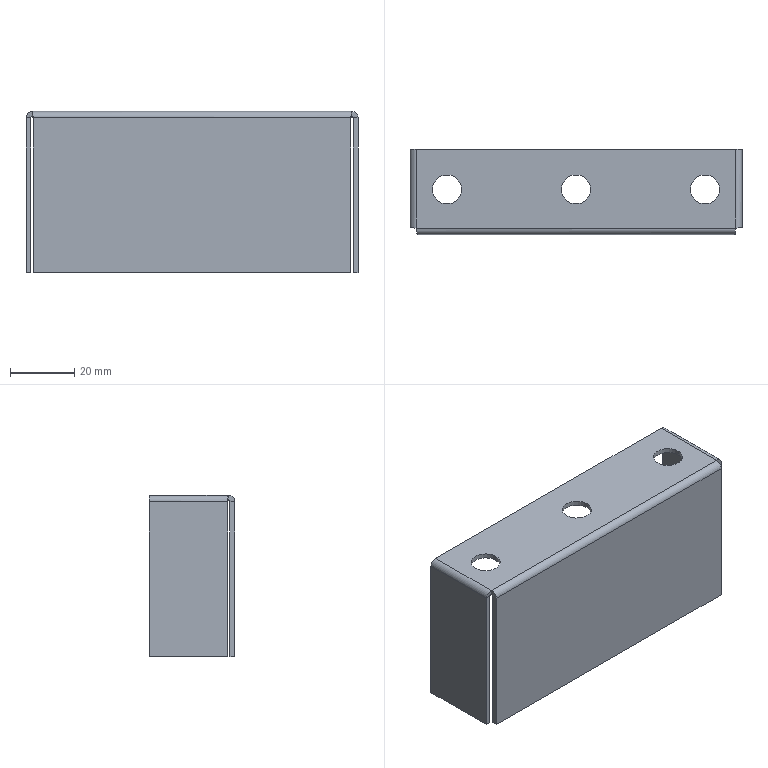Part | SolidWorks | features BaseBody 1 | 1 solid | 36 faces | box 103 x 26.5 x 50 mm | volume 14383 mm3 | plane 20 | cylinder 12 | spline 4 | commonest cylinder face diameters 9 x6 1 x3 4 x3
STEP:
#1=CARTESIAN_POINT('',(-44.5,0.,-1.5));
#2=VERTEX_POINT('',#1);
#3=CARTESIAN_POINT('',(-44.5,0.,0.));
#4=VERTEX_POINT('',#3);
#5=CARTESIAN_POINT('',(-44.5,0.,-1.5));
#6=DIRECTION('',(0.,0.,1.));
#7=VECTOR('',#6,1000.);
#8=LINE('',#5,#7);
#9=EDGE_CURVE('',#2,#4,#8,.T.);
#10=ORIENTED_EDGE('',*,*,#9,.F.);
#11=CARTESIAN_POINT('',(-35.5,0.,-1.5));
#12=VERTEX_POINT('',#11);
#13=CARTESIAN_POINT('',(-40.,0.,-1.5));
#14=DIRECTION('',(0.,0.,1.));
#15=DIRECTION('',(1.,0.,0.));
#16=AXIS2_PLACEMENT_3D('',#13,#14,#15);
#17=CIRCLE('',#16,4.5);
#18=EDGE_CURVE('',#12,#2,#17,.T.);
#19=ORIENTED_EDGE('',*,*,#18,.F.);
#20=CARTESIAN_POINT('',(-35.5,0.,0.));
#21=VERTEX_POINT('',#20);
#22=CARTESIAN_POINT('',(-35.5,0.,-1.5));
#23=DIRECTION('',(0.,0.,1.));
#24=VECTOR('',#23,1000.);
#25=LINE('',#22,#24);
#26=EDGE_CURVE('',#12,#21,#25,.T.);
#27=ORIENTED_EDGE('',*,*,#26,.T.);
#28=CARTESIAN_POINT('',(-40.,0.,0.));
#29=DIRECTION('',(0.,0.,1.));
#30=DIRECTION('',(1.,0.,0.));
#31=AXIS2_PLACEMENT_3D('',#28,#29,#30);
#32=CIRCLE('',#31,4.5);
#33=EDGE_CURVE('',#21,#4,#32,.T.);
#34=ORIENTED_EDGE('',*,*,#33,.T.);
#35=EDGE_LOOP('',(#10,#19,#27,#34));
#36=FACE_OUTER_BOUND('',#35,.T.);
#37=CARTESIAN_POINT('',(-40.,0.,-1.5));
#38=DIRECTION('',(0.,0.,1.));
#39=DIRECTION('',(1.,0.,0.));
#40=AXIS2_PLACEMENT_3D('',#37,#38,#39);
#41=CYLINDRICAL_SURFACE('',#40,4.5);
#42=ADVANCED_FACE('',(#36),#41,.F.);
#43=CARTESIAN_POINT('',(-4.5,0.,-1.5));
#44=VERTEX_POINT('',#43);
#45=CARTESIAN_POINT('',(-4.5,0.,0.));
#46=VERTEX_POINT('',#45);
#47=CARTESIAN_POINT('',(-4.5,0.,-1.5));
#48=DIRECTION('',(0.,0.,1.));
#49=VECTOR('',#48,1000.);
#50=LINE('',#47,#49);
#51=EDGE_CURVE('',#44,#46,#50,.T.);
#52=ORIENTED_EDGE('',*,*,#51,.F.);
#53=CARTESIAN_POINT('',(4.5,0.,-1.5));
#54=VERTEX_POINT('',#53);
#55=CARTESIAN_POINT('',(0.,0.,-1.5));
#56=DIRECTION('',(0.,0.,1.));
#57=DIRECTION('',(1.,0.,0.));
#58=AXIS2_PLACEMENT_3D('',#55,#56,#57);
#59=CIRCLE('',#58,4.5);
#60=EDGE_CURVE('',#54,#44,#59,.T.);
#61=ORIENTED_EDGE('',*,*,#60,.F.);
#62=CARTESIAN_POINT('',(4.5,0.,0.));
#63=VERTEX_POINT('',#62);
#64=CARTESIAN_POINT('',(4.5,0.,-1.5));
#65=DIRECTION('',(0.,0.,1.));
#66=VECTOR('',#65,1000.);
#67=LINE('',#64,#66);
#68=EDGE_CURVE('',#54,#63,#67,.T.);
#69=ORIENTED_EDGE('',*,*,#68,.T.);
#70=CARTESIAN_POINT('',(0.,0.,0.));
#71=DIRECTION('',(0.,0.,1.));
#72=DIRECTION('',(1.,0.,0.));
#73=AXIS2_PLACEMENT_3D('',#70,#71,#72);
#74=CIRCLE('',#73,4.5);
#75=EDGE_CURVE('',#63,#46,#74,.T.);
#76=ORIENTED_EDGE('',*,*,#75,.T.);
#77=EDGE_LOOP('',(#52,#61,#69,#76));
#78=FACE_OUTER_BOUND('',#77,.T.);
#79=CARTESIAN_POINT('',(0.,0.,-1.5));
#80=DIRECTION('',(0.,0.,1.));
#81=DIRECTION('',(1.,0.,0.));
#82=AXIS2_PLACEMENT_3D('',#79,#80,#81);
#83=CYLINDRICAL_SURFACE('',#82,4.5);
#84=ADVANCED_FACE('',(#78),#83,.F.);
#85=CARTESIAN_POINT('',(35.5,0.,-1.5));
#86=VERTEX_POINT('',#85);
#87=CARTESIAN_POINT('',(35.5,0.,0.));
#88=VERTEX_POINT('',#87);
#89=CARTESIAN_POINT('',(35.5,0.,-1.5));
#90=DIRECTION('',(0.,0.,1.));
#91=VECTOR('',#90,1000.);
#92=LINE('',#89,#91);
#93=EDGE_CURVE('',#86,#88,#92,.T.);
#94=ORIENTED_EDGE('',*,*,#93,.F.);
#95=CARTESIAN_POINT('',(44.5,0.,-1.5));
#96=VERTEX_POINT('',#95);
#97=CARTESIAN_POINT('',(40.,0.,-1.5));
#98=DIRECTION('',(0.,0.,1.));
#99=DIRECTION('',(-1.,0.,0.));
#100=AXIS2_PLACEMENT_3D('',#97,#98,#99);
#101=CIRCLE('',#100,4.5);
#102=EDGE_CURVE('',#96,#86,#101,.T.);
#103=ORIENTED_EDGE('',*,*,#102,.F.);
#104=CARTESIAN_POINT('',(44.5,0.,0.));
#105=VERTEX_POINT('',#104);
#106=CARTESIAN_POINT('',(44.5,0.,-1.5));
#107=DIRECTION('',(0.,0.,1.));
#108=VECTOR('',#107,1000.);
#109=LINE('',#106,#108);
#110=EDGE_CURVE('',#96,#105,#109,.T.);
#111=ORIENTED_EDGE('',*,*,#110,.T.);
#112=CARTESIAN_POINT('',(40.,0.,0.));
#113=DIRECTION('',(0.,0.,1.));
#114=DIRECTION('',(-1.,0.,0.));
#115=AXIS2_PLACEMENT_3D('',#112,#113,#114);
#116=CIRCLE('',#115,4.5);
#117=EDGE_CURVE('',#105,#88,#116,.T.);
#118=ORIENTED_EDGE('',*,*,#117,.T.);
#119=EDGE_LOOP('',(#94,#103,#111,#118));
#120=FACE_OUTER_BOUND('',#119,.T.);
#121=CARTESIAN_POINT('',(40.,0.,-1.5));
#122=DIRECTION('',(0.,0.,1.));
#123=DIRECTION('',(1.,0.,0.));
#124=AXIS2_PLACEMENT_3D('',#121,#122,#123);
#125=CYLINDRICAL_SURFACE('',#124,4.5);
#126=ADVANCED_FACE('',(#120),#125,.F.);
#127=CARTESIAN_POINT('',(51.5,-11.793,-50.));
#128=VERTEX_POINT('',#127);
#129=CARTESIAN_POINT('',(50.,-11.793,-50.));
#130=VERTEX_POINT('',#129);
#131=CARTESIAN_POINT('',(51.5,-11.793,-50.));
#132=DIRECTION('',(-1.,0.,0.));
#133=VECTOR('',#132,1000.);
#134=LINE('',#131,#133);
#135=EDGE_CURVE('',#128,#130,#134,.T.);
#136=ORIENTED_EDGE('',*,*,#135,.F.);
#137=CARTESIAN_POINT('',(51.5,-11.793,-2.));
#138=VERTEX_POINT('',#137);
#139=CARTESIAN_POINT('',(51.5,-11.793,0.));
#140=DIRECTION('',(0.,0.,-1.));
#141=VECTOR('',#140,1000.);
#142=LINE('',#139,#141);
#143=EDGE_CURVE('',#138,#128,#142,.T.);
#144=ORIENTED_EDGE('',*,*,#143,.F.);
#145=CARTESIAN_POINT('',(50.,-11.793,-2.));
#146=VERTEX_POINT('',#145);
#147=CARTESIAN_POINT('',(50.,-11.793,-2.));
#148=DIRECTION('',(-1.,0.,0.));
#149=VECTOR('',#148,1000.);
#150=LINE('',#147,#149);
#151=EDGE_CURVE('',#138,#146,#150,.T.);
#152=ORIENTED_EDGE('',*,*,#151,.T.);
#153=CARTESIAN_POINT('',(50.,-11.793,-1.5));
#154=DIRECTION('',(0.,0.,-1.));
#155=VECTOR('',#154,1000.);
#156=LINE('',#153,#155);
#157=EDGE_CURVE('',#146,#130,#156,.T.);
#158=ORIENTED_EDGE('',*,*,#157,.T.);
#159=EDGE_LOOP('',(#136,#144,#152,#158));
#160=FACE_OUTER_BOUND('',#159,.T.);
#161=CARTESIAN_POINT('',(50.,-11.793,-1.5));
#162=DIRECTION('',(0.,1.,0.));
#163=DIRECTION('',(0.,0.,-1.));
#164=AXIS2_PLACEMENT_3D('',#161,#162,#163);
#165=PLANE('',#164);
#166=ADVANCED_FACE('',(#160),#165,.F.);
#167=CARTESIAN_POINT('',(51.5,12.5,-50.));
#168=VERTEX_POINT('',#167);
#169=CARTESIAN_POINT('',(51.5,12.5,-50.));
#170=DIRECTION('',(0.,1.,0.));
#171=VECTOR('',#170,1000.);
#172=LINE('',#169,#171);
#173=EDGE_CURVE('',#128,#168,#172,.T.);
#174=ORIENTED_EDGE('',*,*,#173,.F.);
#175=ORIENTED_EDGE('',*,*,#135,.T.);
#176=CARTESIAN_POINT('',(50.,12.5,-50.));
#177=VERTEX_POINT('',#176);
#178=CARTESIAN_POINT('',(50.,12.5,-50.));
#179=DIRECTION('',(0.,1.,0.));
#180=VECTOR('',#179,1000.);
#181=LINE('',#178,#180);
#182=EDGE_CURVE('',#130,#177,#181,.T.);
#183=ORIENTED_EDGE('',*,*,#182,.T.);
#184=CARTESIAN_POINT('',(51.5,12.5,-50.));
#185=DIRECTION('',(-1.,0.,0.));
#186=VECTOR('',#185,1000.);
#187=LINE('',#184,#186);
#188=EDGE_CURVE('',#168,#177,#187,.T.);
#189=ORIENTED_EDGE('',*,*,#188,.F.);
#190=EDGE_LOOP('',(#174,#175,#183,#189));
#191=FACE_OUTER_BOUND('',#190,.T.);
#192=CARTESIAN_POINT('',(51.5,12.5,-50.));
#193=DIRECTION('',(0.,0.,1.));
#194=DIRECTION('',(1.,0.,0.));
#195=AXIS2_PLACEMENT_3D('',#192,#193,#194);
#196=PLANE('',#195);
#197=ADVANCED_FACE('',(#191),#196,.F.);
#198=ORIENTED_EDGE('',*,*,#157,.F.);
#199=CARTESIAN_POINT('',(50.,12.5,-2.));
#200=VERTEX_POINT('',#199);
#201=CARTESIAN_POINT('',(50.,12.5,-2.));
#202=DIRECTION('',(0.,-1.,0.));
#203=VECTOR('',#202,1000.);
#204=LINE('',#201,#203);
#205=EDGE_CURVE('',#200,#146,#204,.T.);
#206=ORIENTED_EDGE('',*,*,#205,.F.);
#207=CARTESIAN_POINT('',(50.,12.5,-1.5));
#208=DIRECTION('',(0.,0.,1.));
#209=VECTOR('',#208,1000.);
#210=LINE('',#207,#209);
#211=EDGE_CURVE('',#177,#200,#210,.T.);
#212=ORIENTED_EDGE('',*,*,#211,.F.);
#213=ORIENTED_EDGE('',*,*,#182,.F.);
#214=EDGE_LOOP('',(#198,#206,#212,#213));
#215=FACE_OUTER_BOUND('',#214,.T.);
#216=CARTESIAN_POINT('',(50.,0.,0.));
#217=DIRECTION('',(-1.,0.,0.));
#218=DIRECTION('',(0.,0.,1.));
#219=AXIS2_PLACEMENT_3D('',#216,#217,#218);
#220=PLANE('',#219);
#221=ADVANCED_FACE('',(#215),#220,.T.);
#222=CARTESIAN_POINT('',(51.5,12.5,-2.));
#223=VERTEX_POINT('',#222);
#224=CARTESIAN_POINT('',(51.5,0.,-2.));
#225=DIRECTION('',(0.,1.,0.));
#226=VECTOR('',#225,1000.);
#227=LINE('',#224,#226);
#228=EDGE_CURVE('',#138,#223,#227,.T.);
#229=ORIENTED_EDGE('',*,*,#228,.F.);
#230=ORIENTED_EDGE('',*,*,#143,.T.);
#231=ORIENTED_EDGE('',*,*,#173,.T.);
#232=CARTESIAN_POINT('',(51.5,12.5,-1.5));
#233=DIRECTION('',(0.,0.,1.));
#234=VECTOR('',#233,1000.);
#235=LINE('',#232,#234);
#236=EDGE_CURVE('',#168,#223,#235,.T.);
#237=ORIENTED_EDGE('',*,*,#236,.T.);
#238=EDGE_LOOP('',(#229,#230,#231,#237));
#239=FACE_OUTER_BOUND('',#238,.T.);
#240=CARTESIAN_POINT('',(51.5,0.,0.));
#241=DIRECTION('',(-1.,0.,0.));
#242=DIRECTION('',(0.,0.,1.));
#243=AXIS2_PLACEMENT_3D('',#240,#241,#242);
#244=PLANE('',#243);
#245=ADVANCED_FACE('',(#239),#244,.F.);
#246=CARTESIAN_POINT('',(50.,12.5,-2.));
#247=DIRECTION('',(1.,0.,0.));
#248=VECTOR('',#247,1000.);
#249=LINE('',#246,#248);
#250=EDGE_CURVE('',#200,#223,#249,.T.);
#251=ORIENTED_EDGE('',*,*,#250,.T.);
#252=ORIENTED_EDGE('',*,*,#236,.F.);
#253=ORIENTED_EDGE('',*,*,#188,.T.);
#254=ORIENTED_EDGE('',*,*,#211,.T.);
#255=EDGE_LOOP('',(#251,#252,#253,#254));
#256=FACE_OUTER_BOUND('',#255,.T.);
#257=CARTESIAN_POINT('',(51.5,12.5,-1.5));
#258=DIRECTION('',(0.,-1.,0.));
#259=DIRECTION('',(0.,0.,-1.));
#260=AXIS2_PLACEMENT_3D('',#257,#258,#259);
#261=PLANE('',#260);
#262=ADVANCED_FACE('',(#256),#261,.F.);
#263=CARTESIAN_POINT('',(49.5,-12.,-1.5));
#264=VERTEX_POINT('',#263);
#265=CARTESIAN_POINT('',(49.5,12.5,-1.5));
#266=VERTEX_POINT('',#265);
#267=CARTESIAN_POINT('',(49.5,-12.,-1.5));
#268=DIRECTION('',(0.,1.,0.));
#269=VECTOR('',#268,1000.);
#270=LINE('',#267,#269);
#271=EDGE_CURVE('',#264,#266,#270,.T.);
#272=ORIENTED_EDGE('',*,*,#271,.T.);
#273=CARTESIAN_POINT('',(49.5,12.5,-2.));
#274=DIRECTION('',(0.,1.,0.));
#275=DIRECTION('',(0.,0.,-1.));
#276=AXIS2_PLACEMENT_3D('',#273,#274,#275);
#277=CIRCLE('',#276,0.5);
#278=EDGE_CURVE('',#266,#200,#277,.T.);
#279=ORIENTED_EDGE('',*,*,#278,.T.);
#280=ORIENTED_EDGE('',*,*,#205,.T.);
#281=CARTESIAN_POINT('',(50.,-11.793,-2.));
#282=CARTESIAN_POINT('',(50.,-11.827,-1.869));
#283=CARTESIAN_POINT('',(49.946,-11.862,-1.739));
#284=CARTESIAN_POINT('',(49.761,-11.931,-1.554));
#285=CARTESIAN_POINT('',(49.631,-11.965,-1.5));
#286=CARTESIAN_POINT('',(49.5,-12.,-1.5));
#287=B_SPLINE_CURVE_WITH_KNOTS('',3,(#281,#282,#283,#284,#285,#286),.UNSPECIFIED.,.F.,.F.,(4,2,4),(0.,0.5,1.),.UNSPECIFIED.);
#288=EDGE_CURVE('',#146,#264,#287,.T.);
#289=ORIENTED_EDGE('',*,*,#288,.T.);
#290=EDGE_LOOP('',(#272,#279,#280,#289));
#291=FACE_OUTER_BOUND('',#290,.T.);
#292=CARTESIAN_POINT('',(49.5,-12.,-2.));
#293=DIRECTION('',(0.,-1.,0.));
#294=DIRECTION('',(1.,0.,0.));
#295=AXIS2_PLACEMENT_3D('',#292,#293,#294);
#296=CYLINDRICAL_SURFACE('',#295,0.5);
#297=ADVANCED_FACE('',(#291),#296,.F.);
#298=CARTESIAN_POINT('',(49.5,-12.,0.));
#299=VERTEX_POINT('',#298);
#300=CARTESIAN_POINT('',(49.5,12.5,0.));
#301=VERTEX_POINT('',#300);
#302=CARTESIAN_POINT('',(49.5,-12.,0.));
#303=DIRECTION('',(0.,1.,0.));
#304=VECTOR('',#303,1000.);
#305=LINE('',#302,#304);
#306=EDGE_CURVE('',#299,#301,#305,.T.);
#307=ORIENTED_EDGE('',*,*,#306,.F.);
#308=CARTESIAN_POINT('',(51.5,-11.793,-2.));
#309=CARTESIAN_POINT('',(51.5,-11.81,-1.738));
#310=CARTESIAN_POINT('',(51.448,-11.827,-1.477));
#311=CARTESIAN_POINT('',(51.248,-11.862,-0.9928));
#312=CARTESIAN_POINT('',(51.099,-11.879,-0.7709));
#313=CARTESIAN_POINT('',(50.729,-11.914,-0.4007));
#314=CARTESIAN_POINT('',(50.507,-11.931,-0.2524));
#315=CARTESIAN_POINT('',(50.023,-11.965,-0.05205));
#316=CARTESIAN_POINT('',(49.762,-11.983,0.));
#317=CARTESIAN_POINT('',(49.5,-12.,0.));
#318=B_SPLINE_CURVE_WITH_KNOTS('',3,(#308,#309,#310,#311,#312,#313,#314,#315,#316,#317),.UNSPECIFIED.,.F.,.F.,(4,2,2,2,4),(0.,0.25,0.5,0.75,1.),.UNSPECIFIED.);
#319=EDGE_CURVE('',#138,#299,#318,.T.);
#320=ORIENTED_EDGE('',*,*,#319,.F.);
#321=ORIENTED_EDGE('',*,*,#228,.T.);
#322=CARTESIAN_POINT('',(49.5,12.5,-2.));
#323=DIRECTION('',(0.,1.,0.));
#324=DIRECTION('',(0.,0.,-1.));
#325=AXIS2_PLACEMENT_3D('',#322,#323,#324);
#326=CIRCLE('',#325,2.);
#327=EDGE_CURVE('',#301,#223,#326,.T.);
#328=ORIENTED_EDGE('',*,*,#327,.F.);
#329=EDGE_LOOP('',(#307,#320,#321,#328));
#330=FACE_OUTER_BOUND('',#329,.T.);
#331=CARTESIAN_POINT('',(49.5,-12.,-2.));
#332=DIRECTION('',(0.,-1.,0.));
#333=DIRECTION('',(1.,0.,0.));
#334=AXIS2_PLACEMENT_3D('',#331,#332,#333);
#335=CYLINDRICAL_SURFACE('',#334,2.);
#336=ADVANCED_FACE('',(#330),#335,.T.);
#337=ORIENTED_EDGE('',*,*,#288,.F.);
#338=ORIENTED_EDGE('',*,*,#151,.F.);
#339=ORIENTED_EDGE('',*,*,#319,.T.);
#340=CARTESIAN_POINT('',(49.5,-12.,-1.5));
#341=DIRECTION('',(0.,0.,1.));
#342=VECTOR('',#341,1000.);
#343=LINE('',#340,#342);
#344=EDGE_CURVE('',#264,#299,#343,.T.);
#345=ORIENTED_EDGE('',*,*,#344,.F.);
#346=EDGE_LOOP('',(#337,#338,#339,#345));
#347=FACE_OUTER_BOUND('',#346,.T.);
#348=CARTESIAN_POINT('',(51.515,-11.793,-2.));
#349=CARTESIAN_POINT('',(51.515,-11.81,-1.736));
#350=CARTESIAN_POINT('',(51.463,-11.827,-1.473));
#351=CARTESIAN_POINT('',(51.261,-11.862,-0.9852));
#352=CARTESIAN_POINT('',(51.111,-11.879,-0.7617));
#353=CARTESIAN_POINT('',(50.738,-11.914,-0.3887));
#354=CARTESIAN_POINT('',(50.515,-11.931,-0.2393));
#355=CARTESIAN_POINT('',(50.027,-11.965,-0.03745));
#356=CARTESIAN_POINT('',(49.764,-11.983,0.015));
#357=CARTESIAN_POINT('',(49.5,-12.,0.015));
#358=CARTESIAN_POINT('',(51.5,-11.793,-2.));
#359=CARTESIAN_POINT('',(51.5,-11.81,-1.738));
#360=CARTESIAN_POINT('',(51.448,-11.827,-1.477));
#361=CARTESIAN_POINT('',(51.248,-11.862,-0.9928));
#362=CARTESIAN_POINT('',(51.099,-11.879,-0.7709));
#363=CARTESIAN_POINT('',(50.729,-11.914,-0.4007));
#364=CARTESIAN_POINT('',(50.507,-11.931,-0.2524));
#365=CARTESIAN_POINT('',(50.023,-11.965,-0.05205));
#366=CARTESIAN_POINT('',(49.762,-11.983,0.));
#367=CARTESIAN_POINT('',(49.5,-12.,0.));
#368=CARTESIAN_POINT('',(50.,-11.793,-2.));
#369=CARTESIAN_POINT('',(50.,-11.81,-1.935));
#370=CARTESIAN_POINT('',(49.987,-11.827,-1.869));
#371=CARTESIAN_POINT('',(49.937,-11.862,-1.748));
#372=CARTESIAN_POINT('',(49.9,-11.879,-1.693));
#373=CARTESIAN_POINT('',(49.807,-11.914,-1.6));
#374=CARTESIAN_POINT('',(49.752,-11.931,-1.563));
#375=CARTESIAN_POINT('',(49.631,-11.965,-1.513));
#376=CARTESIAN_POINT('',(49.565,-11.983,-1.5));
#377=CARTESIAN_POINT('',(49.5,-12.,-1.5));
#378=CARTESIAN_POINT('',(49.985,-11.793,-2.));
#379=CARTESIAN_POINT('',(49.985,-11.81,-1.937));
#380=CARTESIAN_POINT('',(49.972,-11.827,-1.873));
#381=CARTESIAN_POINT('',(49.924,-11.862,-1.756));
#382=CARTESIAN_POINT('',(49.888,-11.879,-1.702));
#383=CARTESIAN_POINT('',(49.798,-11.914,-1.612));
#384=CARTESIAN_POINT('',(49.744,-11.931,-1.576));
#385=CARTESIAN_POINT('',(49.627,-11.965,-1.528));
#386=CARTESIAN_POINT('',(49.563,-11.983,-1.515));
#387=CARTESIAN_POINT('',(49.5,-12.,-1.515));
#388=B_SPLINE_SURFACE_WITH_KNOTS('',1,3,((#348,#349,#350,#351,#352,#353,#354,#355,#356,#357),(#358,#359,#360,#361,#362,#363,#364,#365,#366,#367),(#368,#369,#370,#371,#372,#373,#374,#375,#376,#377),(#378,#379,#380,#381,#382,#383,#384,#385,#386,#387)),.UNSPECIFIED.,.F.,.F.,.F.,(2,1,1,2),(4,2,2,2,4),(-0.01,0.,1.,1.01),(0.,0.25,0.5,0.75,1.),.UNSPECIFIED.);
#389=ADVANCED_FACE('',(#347),#388,.F.);
#390=ORIENTED_EDGE('',*,*,#250,.F.);
#391=ORIENTED_EDGE('',*,*,#278,.F.);
#392=CARTESIAN_POINT('',(49.5,12.5,-1.5));
#393=DIRECTION('',(0.,0.,1.));
#394=VECTOR('',#393,1000.);
#395=LINE('',#392,#394);
#396=EDGE_CURVE('',#266,#301,#395,.T.);
#397=ORIENTED_EDGE('',*,*,#396,.T.);
#398=ORIENTED_EDGE('',*,*,#327,.T.);
#399=EDGE_LOOP('',(#390,#391,#397,#398));
#400=FACE_OUTER_BOUND('',#399,.T.);
#401=CARTESIAN_POINT('',(49.5,12.5,-2.));
#402=DIRECTION('',(0.,1.,0.));
#403=DIRECTION('',(1.,0.,0.));
#404=AXIS2_PLACEMENT_3D('',#401,#402,#403);
#405=PLANE('',#404);
#406=ADVANCED_FACE('',(#400),#405,.T.);
#407=CARTESIAN_POINT('',(-49.293,-14.,-50.));
#408=VERTEX_POINT('',#407);
#409=CARTESIAN_POINT('',(-49.293,-12.5,-50.));
#410=VERTEX_POINT('',#409);
#411=CARTESIAN_POINT('',(-49.293,-14.,-50.));
#412=DIRECTION('',(0.,1.,0.));
#413=VECTOR('',#412,1000.);
#414=LINE('',#411,#413);
#415=EDGE_CURVE('',#408,#410,#414,.T.);
#416=ORIENTED_EDGE('',*,*,#415,.F.);
#417=CARTESIAN_POINT('',(-49.293,-14.,-2.));
#418=VERTEX_POINT('',#417);
#419=CARTESIAN_POINT('',(-49.293,-14.,0.));
#420=DIRECTION('',(0.,0.,-1.));
#421=VECTOR('',#420,1000.);
#422=LINE('',#419,#421);
#423=EDGE_CURVE('',#418,#408,#422,.T.);
#424=ORIENTED_EDGE('',*,*,#423,.F.);
#425=CARTESIAN_POINT('',(-49.293,-12.5,-2.));
#426=VERTEX_POINT('',#425);
#427=CARTESIAN_POINT('',(-49.293,-12.5,-2.));
#428=DIRECTION('',(0.,1.,0.));
#429=VECTOR('',#428,1000.);
#430=LINE('',#427,#429);
#431=EDGE_CURVE('',#418,#426,#430,.T.);
#432=ORIENTED_EDGE('',*,*,#431,.T.);
#433=CARTESIAN_POINT('',(-49.293,-12.5,-1.5));
#434=DIRECTION('',(0.,0.,-1.));
#435=VECTOR('',#434,1000.);
#436=LINE('',#433,#435);
#437=EDGE_CURVE('',#426,#410,#436,.T.);
#438=ORIENTED_EDGE('',*,*,#437,.T.);
#439=EDGE_LOOP('',(#416,#424,#432,#438));
#440=FACE_OUTER_BOUND('',#439,.T.);
#441=CARTESIAN_POINT('',(-49.293,-12.5,-1.5));
#442=DIRECTION('',(1.,0.,0.));
#443=DIRECTION('',(0.,1.,0.));
#444=AXIS2_PLACEMENT_3D('',#441,#442,#443);
#445=PLANE('',#444);
#446=ADVANCED_FACE('',(#440),#445,.F.);
#447=CARTESIAN_POINT('',(49.293,-14.,-50.));
#448=VERTEX_POINT('',#447);
#449=CARTESIAN_POINT('',(49.293,-12.5,-50.));
#450=VERTEX_POINT('',#449);
#451=CARTESIAN_POINT('',(49.293,-14.,-50.));
#452=DIRECTION('',(0.,1.,0.));
#453=VECTOR('',#452,1000.);
#454=LINE('',#451,#453);
#455=EDGE_CURVE('',#448,#450,#454,.T.);
#456=ORIENTED_EDGE('',*,*,#455,.F.);
#457=CARTESIAN_POINT('',(50.,-14.,-50.));
#458=DIRECTION('',(1.,0.,0.));
#459=VECTOR('',#458,1000.);
#460=LINE('',#457,#459);
#461=EDGE_CURVE('',#408,#448,#460,.T.);
#462=ORIENTED_EDGE('',*,*,#461,.F.);
#463=ORIENTED_EDGE('',*,*,#415,.T.);
#464=CARTESIAN_POINT('',(50.,-12.5,-50.));
#465=DIRECTION('',(1.,0.,0.));
#466=VECTOR('',#465,1000.);
#467=LINE('',#464,#466);
#468=EDGE_CURVE('',#410,#450,#467,.T.);
#469=ORIENTED_EDGE('',*,*,#468,.T.);
#470=EDGE_LOOP('',(#456,#462,#463,#469));
#471=FACE_OUTER_BOUND('',#470,.T.);
#472=CARTESIAN_POINT('',(50.,-14.,-50.));
#473=DIRECTION('',(0.,0.,1.));
#474=DIRECTION('',(0.,-1.,0.));
#475=AXIS2_PLACEMENT_3D('',#472,#473,#474);
#476=PLANE('',#475);
#477=ADVANCED_FACE('',(#471),#476,.F.);
#478=CARTESIAN_POINT('',(49.293,-12.5,-2.));
#479=VERTEX_POINT('',#478);
#480=CARTESIAN_POINT('',(50.,-12.5,-2.));
#481=DIRECTION('',(-1.,0.,0.));
#482=VECTOR('',#481,1000.);
#483=LINE('',#480,#482);
#484=EDGE_CURVE('',#479,#426,#483,.T.);
#485=ORIENTED_EDGE('',*,*,#484,.F.);
#486=CARTESIAN_POINT('',(49.293,-12.5,-1.5));
#487=DIRECTION('',(0.,0.,-1.));
#488=VECTOR('',#487,1000.);
#489=LINE('',#486,#488);
#490=EDGE_CURVE('',#479,#450,#489,.T.);
#491=ORIENTED_EDGE('',*,*,#490,.T.);
#492=ORIENTED_EDGE('',*,*,#468,.F.);
#493=ORIENTED_EDGE('',*,*,#437,.F.);
#494=EDGE_LOOP('',(#485,#491,#492,#493));
#495=FACE_OUTER_BOUND('',#494,.T.);
#496=CARTESIAN_POINT('',(0.,-12.5,0.));
#497=DIRECTION('',(0.,1.,0.));
#498=DIRECTION('',(0.,0.,-1.));
#499=AXIS2_PLACEMENT_3D('',#496,#497,#498);
#500=PLANE('',#499);
#501=ADVANCED_FACE('',(#495),#500,.T.);
#502=CARTESIAN_POINT('',(49.293,-14.,-2.));
#503=VERTEX_POINT('',#502);
#504=CARTESIAN_POINT('',(49.293,-14.,0.));
#505=DIRECTION('',(0.,0.,-1.));
#506=VECTOR('',#505,1000.);
#507=LINE('',#504,#506);
#508=EDGE_CURVE('',#503,#448,#507,.T.);
#509=ORIENTED_EDGE('',*,*,#508,.F.);
#510=CARTESIAN_POINT('',(0.,-14.,-2.));
#511=DIRECTION('',(1.,0.,0.));
#512=VECTOR('',#511,1000.);
#513=LINE('',#510,#512);
#514=EDGE_CURVE('',#418,#503,#513,.T.);
#515=ORIENTED_EDGE('',*,*,#514,.F.);
#516=ORIENTED_EDGE('',*,*,#423,.T.);
#517=ORIENTED_EDGE('',*,*,#461,.T.);
#518=EDGE_LOOP('',(#509,#515,#516,#517));
#519=FACE_OUTER_BOUND('',#518,.T.);
#520=CARTESIAN_POINT('',(0.,-14.,0.));
#521=DIRECTION('',(0.,1.,0.));
#522=DIRECTION('',(0.,0.,-1.));
#523=AXIS2_PLACEMENT_3D('',#520,#521,#522);
#524=PLANE('',#523);
#525=ADVANCED_FACE('',(#519),#524,.F.);
#526=ORIENTED_EDGE('',*,*,#508,.T.);
#527=ORIENTED_EDGE('',*,*,#455,.T.);
#528=ORIENTED_EDGE('',*,*,#490,.F.);
#529=CARTESIAN_POINT('',(49.293,-12.5,-2.));
#530=DIRECTION('',(0.,1.,0.));
#531=VECTOR('',#530,1000.);
#532=LINE('',#529,#531);
#533=EDGE_CURVE('',#503,#479,#532,.T.);
#534=ORIENTED_EDGE('',*,*,#533,.F.);
#535=EDGE_LOOP('',(#526,#527,#528,#534));
#536=FACE_OUTER_BOUND('',#535,.T.);
#537=CARTESIAN_POINT('',(49.293,-12.5,-1.5));
#538=DIRECTION('',(1.,0.,0.));
#539=DIRECTION('',(0.,1.,0.));
#540=AXIS2_PLACEMENT_3D('',#537,#538,#539);
#541=PLANE('',#540);
#542=ADVANCED_FACE('',(#536),#541,.T.);
#543=CARTESIAN_POINT('',(-49.5,-12.,-1.5));
#544=VERTEX_POINT('',#543);
#545=CARTESIAN_POINT('',(-49.5,-12.,-1.5));
#546=DIRECTION('',(1.,0.,0.));
#547=VECTOR('',#546,1000.);
#548=LINE('',#545,#547);
#549=EDGE_CURVE('',#544,#264,#548,.T.);
#550=ORIENTED_EDGE('',*,*,#549,.T.);
#551=CARTESIAN_POINT('',(49.5,-12.,-1.5));
#552=CARTESIAN_POINT('',(49.465,-12.131,-1.5));
#553=CARTESIAN_POINT('',(49.431,-12.261,-1.554));
#554=CARTESIAN_POINT('',(49.362,-12.446,-1.739));
#555=CARTESIAN_POINT('',(49.327,-12.5,-1.869));
#556=CARTESIAN_POINT('',(49.293,-12.5,-2.));
#557=B_SPLINE_CURVE_WITH_KNOTS('',3,(#551,#552,#553,#554,#555,#556),.UNSPECIFIED.,.F.,.F.,(4,2,4),(0.,0.5,1.),.UNSPECIFIED.);
#558=EDGE_CURVE('',#264,#479,#557,.T.);
#559=ORIENTED_EDGE('',*,*,#558,.T.);
#560=ORIENTED_EDGE('',*,*,#484,.T.);
#561=CARTESIAN_POINT('',(-49.293,-12.5,-2.));
#562=CARTESIAN_POINT('',(-49.327,-12.5,-1.869));
#563=CARTESIAN_POINT('',(-49.362,-12.446,-1.739));
#564=CARTESIAN_POINT('',(-49.431,-12.261,-1.554));
#565=CARTESIAN_POINT('',(-49.465,-12.131,-1.5));
#566=CARTESIAN_POINT('',(-49.5,-12.,-1.5));
#567=B_SPLINE_CURVE_WITH_KNOTS('',3,(#561,#562,#563,#564,#565,#566),.UNSPECIFIED.,.F.,.F.,(4,2,4),(0.,0.5,1.),.UNSPECIFIED.);
#568=EDGE_CURVE('',#426,#544,#567,.T.);
#569=ORIENTED_EDGE('',*,*,#568,.T.);
#570=EDGE_LOOP('',(#550,#559,#560,#569));
#571=FACE_OUTER_BOUND('',#570,.T.);
#572=CARTESIAN_POINT('',(-49.5,-12.,-2.));
#573=DIRECTION('',(-1.,0.,0.));
#574=DIRECTION('',(0.,-1.,0.));
#575=AXIS2_PLACEMENT_3D('',#572,#573,#574);
#576=CYLINDRICAL_SURFACE('',#575,0.5);
#577=ADVANCED_FACE('',(#571),#576,.F.);
#578=CARTESIAN_POINT('',(-49.5,-12.,0.));
#579=VERTEX_POINT('',#578);
#580=CARTESIAN_POINT('',(-49.5,-12.,0.));
#581=DIRECTION('',(1.,0.,0.));
#582=VECTOR('',#581,1000.);
#583=LINE('',#580,#582);
#584=EDGE_CURVE('',#579,#299,#583,.T.);
#585=ORIENTED_EDGE('',*,*,#584,.F.);
#586=CARTESIAN_POINT('',(-49.293,-14.,-2.));
#587=CARTESIAN_POINT('',(-49.31,-14.,-1.738));
#588=CARTESIAN_POINT('',(-49.327,-13.948,-1.477));
#589=CARTESIAN_POINT('',(-49.362,-13.748,-0.9928));
#590=CARTESIAN_POINT('',(-49.379,-13.599,-0.7709));
#591=CARTESIAN_POINT('',(-49.414,-13.229,-0.4007));
#592=CARTESIAN_POINT('',(-49.431,-13.007,-0.2524));
#593=CARTESIAN_POINT('',(-49.465,-12.523,-0.05205));
#594=CARTESIAN_POINT('',(-49.483,-12.262,0.));
#595=CARTESIAN_POINT('',(-49.5,-12.,0.));
#596=B_SPLINE_CURVE_WITH_KNOTS('',3,(#586,#587,#588,#589,#590,#591,#592,#593,#594,#595),.UNSPECIFIED.,.F.,.F.,(4,2,2,2,4),(0.,0.25,0.5,0.75,1.),.UNSPECIFIED.);
#597=EDGE_CURVE('',#418,#579,#596,.T.);
#598=ORIENTED_EDGE('',*,*,#597,.F.);
#599=ORIENTED_EDGE('',*,*,#514,.T.);
#600=CARTESIAN_POINT('',(49.5,-12.,0.));
#601=CARTESIAN_POINT('',(49.483,-12.262,0.));
#602=CARTESIAN_POINT('',(49.465,-12.523,-0.05205));
#603=CARTESIAN_POINT('',(49.431,-13.007,-0.2524));
#604=CARTESIAN_POINT('',(49.414,-13.229,-0.4007));
#605=CARTESIAN_POINT('',(49.379,-13.599,-0.7709));
#606=CARTESIAN_POINT('',(49.362,-13.748,-0.9928));
#607=CARTESIAN_POINT('',(49.327,-13.948,-1.477));
#608=CARTESIAN_POINT('',(49.31,-14.,-1.738));
#609=CARTESIAN_POINT('',(49.293,-14.,-2.));
#610=B_SPLINE_CURVE_WITH_KNOTS('',3,(#600,#601,#602,#603,#604,#605,#606,#607,#608,#609),.UNSPECIFIED.,.F.,.F.,(4,2,2,2,4),(0.,0.25,0.5,0.75,1.),.UNSPECIFIED.);
#611=EDGE_CURVE('',#299,#503,#610,.T.);
#612=ORIENTED_EDGE('',*,*,#611,.F.);
#613=EDGE_LOOP('',(#585,#598,#599,#612));
#614=FACE_OUTER_BOUND('',#613,.T.);
#615=CARTESIAN_POINT('',(-49.5,-12.,-2.));
#616=DIRECTION('',(-1.,0.,0.));
#617=DIRECTION('',(0.,-1.,0.));
#618=AXIS2_PLACEMENT_3D('',#615,#616,#617);
#619=CYLINDRICAL_SURFACE('',#618,2.);
#620=ADVANCED_FACE('',(#614),#619,.T.);
#621=ORIENTED_EDGE('',*,*,#568,.F.);
#622=ORIENTED_EDGE('',*,*,#431,.F.);
#623=ORIENTED_EDGE('',*,*,#597,.T.);
#624=CARTESIAN_POINT('',(-49.5,-12.,-1.5));
#625=DIRECTION('',(0.,0.,1.));
#626=VECTOR('',#625,1000.);
#627=LINE('',#624,#626);
#628=EDGE_CURVE('',#544,#579,#627,.T.);
#629=ORIENTED_EDGE('',*,*,#628,.F.);
#630=EDGE_LOOP('',(#621,#622,#623,#629));
#631=FACE_OUTER_BOUND('',#630,.T.);
#632=CARTESIAN_POINT('',(-49.293,-14.015,-2.));
#633=CARTESIAN_POINT('',(-49.31,-14.015,-1.736));
#634=CARTESIAN_POINT('',(-49.327,-13.963,-1.473));
#635=CARTESIAN_POINT('',(-49.362,-13.761,-0.9852));
#636=CARTESIAN_POINT('',(-49.379,-13.611,-0.7617));
#637=CARTESIAN_POINT('',(-49.414,-13.238,-0.3887));
#638=CARTESIAN_POINT('',(-49.431,-13.015,-0.2393));
#639=CARTESIAN_POINT('',(-49.465,-12.527,-0.03745));
#640=CARTESIAN_POINT('',(-49.483,-12.264,0.015));
#641=CARTESIAN_POINT('',(-49.5,-12.,0.015));
#642=CARTESIAN_POINT('',(-49.293,-14.,-2.));
#643=CARTESIAN_POINT('',(-49.31,-14.,-1.738));
#644=CARTESIAN_POINT('',(-49.327,-13.948,-1.477));
#645=CARTESIAN_POINT('',(-49.362,-13.748,-0.9928));
#646=CARTESIAN_POINT('',(-49.379,-13.599,-0.7709));
#647=CARTESIAN_POINT('',(-49.414,-13.229,-0.4007));
#648=CARTESIAN_POINT('',(-49.431,-13.007,-0.2524));
#649=CARTESIAN_POINT('',(-49.465,-12.523,-0.05205));
#650=CARTESIAN_POINT('',(-49.483,-12.262,0.));
#651=CARTESIAN_POINT('',(-49.5,-12.,0.));
#652=CARTESIAN_POINT('',(-49.293,-12.5,-2.));
#653=CARTESIAN_POINT('',(-49.31,-12.5,-1.935));
#654=CARTESIAN_POINT('',(-49.327,-12.487,-1.869));
#655=CARTESIAN_POINT('',(-49.362,-12.437,-1.748));
#656=CARTESIAN_POINT('',(-49.379,-12.4,-1.693));
#657=CARTESIAN_POINT('',(-49.414,-12.307,-1.6));
#658=CARTESIAN_POINT('',(-49.431,-12.252,-1.563));
#659=CARTESIAN_POINT('',(-49.465,-12.131,-1.513));
#660=CARTESIAN_POINT('',(-49.483,-12.065,-1.5));
#661=CARTESIAN_POINT('',(-49.5,-12.,-1.5));
#662=CARTESIAN_POINT('',(-49.293,-12.485,-2.));
#663=CARTESIAN_POINT('',(-49.31,-12.485,-1.937));
#664=CARTESIAN_POINT('',(-49.327,-12.472,-1.873));
#665=CARTESIAN_POINT('',(-49.362,-12.424,-1.756));
#666=CARTESIAN_POINT('',(-49.379,-12.388,-1.702));
#667=CARTESIAN_POINT('',(-49.414,-12.298,-1.612));
#668=CARTESIAN_POINT('',(-49.431,-12.244,-1.576));
#669=CARTESIAN_POINT('',(-49.465,-12.127,-1.528));
#670=CARTESIAN_POINT('',(-49.483,-12.063,-1.515));
#671=CARTESIAN_POINT('',(-49.5,-12.,-1.515));
#672=B_SPLINE_SURFACE_WITH_KNOTS('',1,3,((#632,#633,#634,#635,#636,#637,#638,#639,#640,#641),(#642,#643,#644,#645,#646,#647,#648,#649,#650,#651),(#652,#653,#654,#655,#656,#657,#658,#659,#660,#661),(#662,#663,#664,#665,#666,#667,#668,#669,#670,#671)),.UNSPECIFIED.,.F.,.F.,.F.,(2,1,1,2),(4,2,2,2,4),(-0.01,0.,1.,1.01),(0.,0.25,0.5,0.75,1.),.UNSPECIFIED.);
#673=ADVANCED_FACE('',(#631),#672,.F.);
#674=ORIENTED_EDGE('',*,*,#533,.T.);
#675=ORIENTED_EDGE('',*,*,#558,.F.);
#676=ORIENTED_EDGE('',*,*,#344,.T.);
#677=ORIENTED_EDGE('',*,*,#611,.T.);
#678=EDGE_LOOP('',(#674,#675,#676,#677));
#679=FACE_OUTER_BOUND('',#678,.T.);
#680=CARTESIAN_POINT('',(49.5,-12.,0.015));
#681=CARTESIAN_POINT('',(49.483,-12.264,0.015));
#682=CARTESIAN_POINT('',(49.465,-12.527,-0.03745));
#683=CARTESIAN_POINT('',(49.431,-13.015,-0.2393));
#684=CARTESIAN_POINT('',(49.414,-13.238,-0.3887));
#685=CARTESIAN_POINT('',(49.379,-13.611,-0.7617));
#686=CARTESIAN_POINT('',(49.362,-13.761,-0.9852));
#687=CARTESIAN_POINT('',(49.327,-13.963,-1.473));
#688=CARTESIAN_POINT('',(49.31,-14.015,-1.736));
#689=CARTESIAN_POINT('',(49.293,-14.015,-2.));
#690=CARTESIAN_POINT('',(49.5,-12.,0.));
#691=CARTESIAN_POINT('',(49.483,-12.262,0.));
#692=CARTESIAN_POINT('',(49.465,-12.523,-0.05205));
#693=CARTESIAN_POINT('',(49.431,-13.007,-0.2524));
#694=CARTESIAN_POINT('',(49.414,-13.229,-0.4007));
#695=CARTESIAN_POINT('',(49.379,-13.599,-0.7709));
#696=CARTESIAN_POINT('',(49.362,-13.748,-0.9928));
#697=CARTESIAN_POINT('',(49.327,-13.948,-1.477));
#698=CARTESIAN_POINT('',(49.31,-14.,-1.738));
#699=CARTESIAN_POINT('',(49.293,-14.,-2.));
#700=CARTESIAN_POINT('',(49.5,-12.,-1.5));
#701=CARTESIAN_POINT('',(49.483,-12.065,-1.5));
#702=CARTESIAN_POINT('',(49.465,-12.131,-1.513));
#703=CARTESIAN_POINT('',(49.431,-12.252,-1.563));
#704=CARTESIAN_POINT('',(49.414,-12.307,-1.6));
#705=CARTESIAN_POINT('',(49.379,-12.4,-1.693));
#706=CARTESIAN_POINT('',(49.362,-12.437,-1.748));
#707=CARTESIAN_POINT('',(49.327,-12.487,-1.869));
#708=CARTESIAN_POINT('',(49.31,-12.5,-1.935));
#709=CARTESIAN_POINT('',(49.293,-12.5,-2.));
#710=CARTESIAN_POINT('',(49.5,-12.,-1.515));
#711=CARTESIAN_POINT('',(49.483,-12.063,-1.515));
#712=CARTESIAN_POINT('',(49.465,-12.127,-1.528));
#713=CARTESIAN_POINT('',(49.431,-12.244,-1.576));
#714=CARTESIAN_POINT('',(49.414,-12.298,-1.612));
#715=CARTESIAN_POINT('',(49.379,-12.388,-1.702));
#716=CARTESIAN_POINT('',(49.362,-12.424,-1.756));
#717=CARTESIAN_POINT('',(49.327,-12.472,-1.873));
#718=CARTESIAN_POINT('',(49.31,-12.485,-1.937));
#719=CARTESIAN_POINT('',(49.293,-12.485,-2.));
#720=B_SPLINE_SURFACE_WITH_KNOTS('',1,3,((#680,#681,#682,#683,#684,#685,#686,#687,#688,#689),(#690,#691,#692,#693,#694,#695,#696,#697,#698,#699),(#700,#701,#702,#703,#704,#705,#706,#707,#708,#709),(#710,#711,#712,#713,#714,#715,#716,#717,#718,#719)),.UNSPECIFIED.,.F.,.F.,.F.,(2,1,1,2),(4,2,2,2,4),(-0.01,0.,1.,1.01),(0.,0.25,0.5,0.75,1.),.UNSPECIFIED.);
#721=ADVANCED_FACE('',(#679),#720,.F.);
#722=CARTESIAN_POINT('',(-50.,12.5,-2.));
#723=VERTEX_POINT('',#722);
#724=CARTESIAN_POINT('',(-51.5,12.5,-2.));
#725=VERTEX_POINT('',#724);
#726=CARTESIAN_POINT('',(-50.,12.5,-2.));
#727=DIRECTION('',(-1.,0.,0.));
#728=VECTOR('',#727,1000.);
#729=LINE('',#726,#728);
#730=EDGE_CURVE('',#723,#725,#729,.T.);
#731=ORIENTED_EDGE('',*,*,#730,.F.);
#732=CARTESIAN_POINT('',(-50.,12.5,-50.));
#733=VERTEX_POINT('',#732);
#734=CARTESIAN_POINT('',(-50.,12.5,-50.));
#735=DIRECTION('',(0.,0.,-1.));
#736=VECTOR('',#735,1000.);
#737=LINE('',#734,#736);
#738=EDGE_CURVE('',#723,#733,#737,.T.);
#739=ORIENTED_EDGE('',*,*,#738,.T.);
#740=CARTESIAN_POINT('',(-51.5,12.5,-50.));
#741=VERTEX_POINT('',#740);
#742=CARTESIAN_POINT('',(-51.5,12.5,-50.));
#743=DIRECTION('',(1.,0.,0.));
#744=VECTOR('',#743,1000.);
#745=LINE('',#742,#744);
#746=EDGE_CURVE('',#741,#733,#745,.T.);
#747=ORIENTED_EDGE('',*,*,#746,.F.);
#748=CARTESIAN_POINT('',(-51.5,12.5,-50.));
#749=DIRECTION('',(0.,0.,-1.));
#750=VECTOR('',#749,1000.);
#751=LINE('',#748,#750);
#752=EDGE_CURVE('',#725,#741,#751,.T.);
#753=ORIENTED_EDGE('',*,*,#752,.F.);
#754=EDGE_LOOP('',(#731,#739,#747,#753));
#755=FACE_OUTER_BOUND('',#754,.T.);
#756=CARTESIAN_POINT('',(-51.5,12.5,-50.));
#757=DIRECTION('',(0.,-1.,0.));
#758=DIRECTION('',(-1.,0.,0.));
#759=AXIS2_PLACEMENT_3D('',#756,#757,#758);
#760=PLANE('',#759);
#761=ADVANCED_FACE('',(#755),#760,.F.);
#762=CARTESIAN_POINT('',(-51.5,-11.793,-50.));
#763=VERTEX_POINT('',#762);
#764=CARTESIAN_POINT('',(-50.,-11.793,-50.));
#765=VERTEX_POINT('',#764);
#766=CARTESIAN_POINT('',(-51.5,-11.793,-50.));
#767=DIRECTION('',(1.,0.,0.));
#768=VECTOR('',#767,1000.);
#769=LINE('',#766,#768);
#770=EDGE_CURVE('',#763,#765,#769,.T.);
#771=ORIENTED_EDGE('',*,*,#770,.F.);
#772=CARTESIAN_POINT('',(-51.5,-12.5,-50.));
#773=DIRECTION('',(0.,-1.,0.));
#774=VECTOR('',#773,1000.);
#775=LINE('',#772,#774);
#776=EDGE_CURVE('',#741,#763,#775,.T.);
#777=ORIENTED_EDGE('',*,*,#776,.F.);
#778=ORIENTED_EDGE('',*,*,#746,.T.);
#779=CARTESIAN_POINT('',(-50.,-12.5,-50.));
#780=DIRECTION('',(0.,-1.,0.));
#781=VECTOR('',#780,1000.);
#782=LINE('',#779,#781);
#783=EDGE_CURVE('',#733,#765,#782,.T.);
#784=ORIENTED_EDGE('',*,*,#783,.T.);
#785=EDGE_LOOP('',(#771,#777,#778,#784));
#786=FACE_OUTER_BOUND('',#785,.T.);
#787=CARTESIAN_POINT('',(-51.5,-12.5,-50.));
#788=DIRECTION('',(0.,0.,1.));
#789=DIRECTION('',(1.,0.,0.));
#790=AXIS2_PLACEMENT_3D('',#787,#788,#789);
#791=PLANE('',#790);
#792=ADVANCED_FACE('',(#786),#791,.F.);
#793=CARTESIAN_POINT('',(-50.,-11.793,-2.));
#794=VERTEX_POINT('',#793);
#795=CARTESIAN_POINT('',(-50.,-12.5,-2.));
#796=DIRECTION('',(0.,1.,0.));
#797=VECTOR('',#796,1000.);
#798=LINE('',#795,#797);
#799=EDGE_CURVE('',#794,#723,#798,.T.);
#800=ORIENTED_EDGE('',*,*,#799,.F.);
#801=CARTESIAN_POINT('',(-50.,-11.793,-1.5));
#802=DIRECTION('',(0.,0.,-1.));
#803=VECTOR('',#802,1000.);
#804=LINE('',#801,#803);
#805=EDGE_CURVE('',#794,#765,#804,.T.);
#806=ORIENTED_EDGE('',*,*,#805,.T.);
#807=ORIENTED_EDGE('',*,*,#783,.F.);
#808=ORIENTED_EDGE('',*,*,#738,.F.);
#809=EDGE_LOOP('',(#800,#806,#807,#808));
#810=FACE_OUTER_BOUND('',#809,.T.);
#811=CARTESIAN_POINT('',(-50.,0.,0.));
#812=DIRECTION('',(1.,0.,0.));
#813=DIRECTION('',(0.,0.,-1.));
#814=AXIS2_PLACEMENT_3D('',#811,#812,#813);
#815=PLANE('',#814);
#816=ADVANCED_FACE('',(#810),#815,.T.);
#817=CARTESIAN_POINT('',(-51.5,-11.793,-2.));
#818=VERTEX_POINT('',#817);
#819=CARTESIAN_POINT('',(-51.5,-11.793,0.));
#820=DIRECTION('',(0.,0.,-1.));
#821=VECTOR('',#820,1000.);
#822=LINE('',#819,#821);
#823=EDGE_CURVE('',#818,#763,#822,.T.);
#824=ORIENTED_EDGE('',*,*,#823,.F.);
#825=CARTESIAN_POINT('',(-51.5,0.,-2.));
#826=DIRECTION('',(0.,-1.,0.));
#827=VECTOR('',#826,1000.);
#828=LINE('',#825,#827);
#829=EDGE_CURVE('',#725,#818,#828,.T.);
#830=ORIENTED_EDGE('',*,*,#829,.F.);
#831=ORIENTED_EDGE('',*,*,#752,.T.);
#832=ORIENTED_EDGE('',*,*,#776,.T.);
#833=EDGE_LOOP('',(#824,#830,#831,#832));
#834=FACE_OUTER_BOUND('',#833,.T.);
#835=CARTESIAN_POINT('',(-51.5,0.,0.));
#836=DIRECTION('',(1.,0.,0.));
#837=DIRECTION('',(0.,0.,-1.));
#838=AXIS2_PLACEMENT_3D('',#835,#836,#837);
#839=PLANE('',#838);
#840=ADVANCED_FACE('',(#834),#839,.F.);
#841=ORIENTED_EDGE('',*,*,#823,.T.);
#842=ORIENTED_EDGE('',*,*,#770,.T.);
#843=ORIENTED_EDGE('',*,*,#805,.F.);
#844=CARTESIAN_POINT('',(-50.,-11.793,-2.));
#845=DIRECTION('',(1.,0.,0.));
#846=VECTOR('',#845,1000.);
#847=LINE('',#844,#846);
#848=EDGE_CURVE('',#818,#794,#847,.T.);
#849=ORIENTED_EDGE('',*,*,#848,.F.);
#850=EDGE_LOOP('',(#841,#842,#843,#849));
#851=FACE_OUTER_BOUND('',#850,.T.);
#852=CARTESIAN_POINT('',(-50.,-11.793,-1.5));
#853=DIRECTION('',(0.,-1.,0.));
#854=DIRECTION('',(0.,0.,-1.));
#855=AXIS2_PLACEMENT_3D('',#852,#853,#854);
#856=PLANE('',#855);
#857=ADVANCED_FACE('',(#851),#856,.T.);
#858=CARTESIAN_POINT('',(-49.5,12.5,-1.5));
#859=VERTEX_POINT('',#858);
#860=CARTESIAN_POINT('',(-49.5,12.5,-1.5));
#861=DIRECTION('',(0.,-1.,0.));
#862=VECTOR('',#861,1000.);
#863=LINE('',#860,#862);
#864=EDGE_CURVE('',#859,#544,#863,.T.);
#865=ORIENTED_EDGE('',*,*,#864,.T.);
#866=CARTESIAN_POINT('',(-49.5,-12.,-1.5));
#867=CARTESIAN_POINT('',(-49.631,-11.965,-1.5));
#868=CARTESIAN_POINT('',(-49.761,-11.931,-1.554));
#869=CARTESIAN_POINT('',(-49.946,-11.862,-1.739));
#870=CARTESIAN_POINT('',(-50.,-11.827,-1.869));
#871=CARTESIAN_POINT('',(-50.,-11.793,-2.));
#872=B_SPLINE_CURVE_WITH_KNOTS('',3,(#866,#867,#868,#869,#870,#871),.UNSPECIFIED.,.F.,.F.,(4,2,4),(0.,0.5,1.),.UNSPECIFIED.);
#873=EDGE_CURVE('',#544,#794,#872,.T.);
#874=ORIENTED_EDGE('',*,*,#873,.T.);
#875=ORIENTED_EDGE('',*,*,#799,.T.);
#876=CARTESIAN_POINT('',(-49.5,12.5,-2.));
#877=DIRECTION('',(0.,1.,0.));
#878=DIRECTION('',(0.,0.,1.));
#879=AXIS2_PLACEMENT_3D('',#876,#877,#878);
#880=CIRCLE('',#879,0.5);
#881=EDGE_CURVE('',#723,#859,#880,.T.);
#882=ORIENTED_EDGE('',*,*,#881,.T.);
#883=EDGE_LOOP('',(#865,#874,#875,#882));
#884=FACE_OUTER_BOUND('',#883,.T.);
#885=CARTESIAN_POINT('',(-49.5,12.5,-2.));
#886=DIRECTION('',(0.,1.,0.));
#887=DIRECTION('',(-1.,0.,0.));
#888=AXIS2_PLACEMENT_3D('',#885,#886,#887);
#889=CYLINDRICAL_SURFACE('',#888,0.5);
#890=ADVANCED_FACE('',(#884),#889,.F.);
#891=CARTESIAN_POINT('',(-49.5,12.5,0.));
#892=VERTEX_POINT('',#891);
#893=CARTESIAN_POINT('',(-49.5,12.5,0.));
#894=DIRECTION('',(0.,-1.,0.));
#895=VECTOR('',#894,1000.);
#896=LINE('',#893,#895);
#897=EDGE_CURVE('',#892,#579,#896,.T.);
#898=ORIENTED_EDGE('',*,*,#897,.F.);
#899=CARTESIAN_POINT('',(-49.5,12.5,-2.));
#900=DIRECTION('',(0.,1.,0.));
#901=DIRECTION('',(0.,0.,1.));
#902=AXIS2_PLACEMENT_3D('',#899,#900,#901);
#903=CIRCLE('',#902,2.);
#904=EDGE_CURVE('',#725,#892,#903,.T.);
#905=ORIENTED_EDGE('',*,*,#904,.F.);
#906=ORIENTED_EDGE('',*,*,#829,.T.);
#907=CARTESIAN_POINT('',(-49.5,-12.,0.));
#908=CARTESIAN_POINT('',(-49.762,-11.983,0.));
#909=CARTESIAN_POINT('',(-50.023,-11.965,-0.05205));
#910=CARTESIAN_POINT('',(-50.507,-11.931,-0.2524));
#911=CARTESIAN_POINT('',(-50.729,-11.914,-0.4007));
#912=CARTESIAN_POINT('',(-51.099,-11.879,-0.7709));
#913=CARTESIAN_POINT('',(-51.248,-11.862,-0.9928));
#914=CARTESIAN_POINT('',(-51.448,-11.827,-1.477));
#915=CARTESIAN_POINT('',(-51.5,-11.81,-1.738));
#916=CARTESIAN_POINT('',(-51.5,-11.793,-2.));
#917=B_SPLINE_CURVE_WITH_KNOTS('',3,(#907,#908,#909,#910,#911,#912,#913,#914,#915,#916),.UNSPECIFIED.,.F.,.F.,(4,2,2,2,4),(0.,0.25,0.5,0.75,1.),.UNSPECIFIED.);
#918=EDGE_CURVE('',#579,#818,#917,.T.);
#919=ORIENTED_EDGE('',*,*,#918,.F.);
#920=EDGE_LOOP('',(#898,#905,#906,#919));
#921=FACE_OUTER_BOUND('',#920,.T.);
#922=CARTESIAN_POINT('',(-49.5,12.5,-2.));
#923=DIRECTION('',(0.,1.,0.));
#924=DIRECTION('',(-1.,0.,0.));
#925=AXIS2_PLACEMENT_3D('',#922,#923,#924);
#926=CYLINDRICAL_SURFACE('',#925,2.);
#927=ADVANCED_FACE('',(#921),#926,.T.);
#928=ORIENTED_EDGE('',*,*,#881,.F.);
#929=ORIENTED_EDGE('',*,*,#730,.T.);
#930=ORIENTED_EDGE('',*,*,#904,.T.);
#931=CARTESIAN_POINT('',(-49.5,12.5,-1.5));
#932=DIRECTION('',(0.,0.,1.));
#933=VECTOR('',#932,1000.);
#934=LINE('',#931,#933);
#935=EDGE_CURVE('',#859,#892,#934,.T.);
#936=ORIENTED_EDGE('',*,*,#935,.F.);
#937=EDGE_LOOP('',(#928,#929,#930,#936));
#938=FACE_OUTER_BOUND('',#937,.T.);
#939=CARTESIAN_POINT('',(-49.5,12.5,-2.));
#940=DIRECTION('',(0.,-1.,0.));
#941=DIRECTION('',(0.,0.,-1.));
#942=AXIS2_PLACEMENT_3D('',#939,#940,#941);
#943=PLANE('',#942);
#944=ADVANCED_FACE('',(#938),#943,.F.);
#945=ORIENTED_EDGE('',*,*,#848,.T.);
#946=ORIENTED_EDGE('',*,*,#873,.F.);
#947=ORIENTED_EDGE('',*,*,#628,.T.);
#948=ORIENTED_EDGE('',*,*,#918,.T.);
#949=EDGE_LOOP('',(#945,#946,#947,#948));
#950=FACE_OUTER_BOUND('',#949,.T.);
#951=CARTESIAN_POINT('',(-49.5,-12.,0.015));
#952=CARTESIAN_POINT('',(-49.764,-11.983,0.015));
#953=CARTESIAN_POINT('',(-50.027,-11.965,-0.03745));
#954=CARTESIAN_POINT('',(-50.515,-11.931,-0.2393));
#955=CARTESIAN_POINT('',(-50.738,-11.914,-0.3887));
#956=CARTESIAN_POINT('',(-51.111,-11.879,-0.7617));
#957=CARTESIAN_POINT('',(-51.261,-11.862,-0.9852));
#958=CARTESIAN_POINT('',(-51.463,-11.827,-1.473));
#959=CARTESIAN_POINT('',(-51.515,-11.81,-1.736));
#960=CARTESIAN_POINT('',(-51.515,-11.793,-2.));
#961=CARTESIAN_POINT('',(-49.5,-12.,0.));
#962=CARTESIAN_POINT('',(-49.762,-11.983,0.));
#963=CARTESIAN_POINT('',(-50.023,-11.965,-0.05205));
#964=CARTESIAN_POINT('',(-50.507,-11.931,-0.2524));
#965=CARTESIAN_POINT('',(-50.729,-11.914,-0.4007));
#966=CARTESIAN_POINT('',(-51.099,-11.879,-0.7709));
#967=CARTESIAN_POINT('',(-51.248,-11.862,-0.9928));
#968=CARTESIAN_POINT('',(-51.448,-11.827,-1.477));
#969=CARTESIAN_POINT('',(-51.5,-11.81,-1.738));
#970=CARTESIAN_POINT('',(-51.5,-11.793,-2.));
#971=CARTESIAN_POINT('',(-49.5,-12.,-1.5));
#972=CARTESIAN_POINT('',(-49.565,-11.983,-1.5));
#973=CARTESIAN_POINT('',(-49.631,-11.965,-1.513));
#974=CARTESIAN_POINT('',(-49.752,-11.931,-1.563));
#975=CARTESIAN_POINT('',(-49.807,-11.914,-1.6));
#976=CARTESIAN_POINT('',(-49.9,-11.879,-1.693));
#977=CARTESIAN_POINT('',(-49.937,-11.862,-1.748));
#978=CARTESIAN_POINT('',(-49.987,-11.827,-1.869));
#979=CARTESIAN_POINT('',(-50.,-11.81,-1.935));
#980=CARTESIAN_POINT('',(-50.,-11.793,-2.));
#981=CARTESIAN_POINT('',(-49.5,-12.,-1.515));
#982=CARTESIAN_POINT('',(-49.563,-11.983,-1.515));
#983=CARTESIAN_POINT('',(-49.627,-11.965,-1.528));
#984=CARTESIAN_POINT('',(-49.744,-11.931,-1.576));
#985=CARTESIAN_POINT('',(-49.798,-11.914,-1.612));
#986=CARTESIAN_POINT('',(-49.888,-11.879,-1.702));
#987=CARTESIAN_POINT('',(-49.924,-11.862,-1.756));
#988=CARTESIAN_POINT('',(-49.972,-11.827,-1.873));
#989=CARTESIAN_POINT('',(-49.985,-11.81,-1.937));
#990=CARTESIAN_POINT('',(-49.985,-11.793,-2.));
#991=B_SPLINE_SURFACE_WITH_KNOTS('',1,3,((#951,#952,#953,#954,#955,#956,#957,#958,#959,#960),(#961,#962,#963,#964,#965,#966,#967,#968,#969,#970),(#971,#972,#973,#974,#975,#976,#977,#978,#979,#980),(#981,#982,#983,#984,#985,#986,#987,#988,#989,#990)),.UNSPECIFIED.,.F.,.F.,.F.,(2,1,1,2),(4,2,2,2,4),(-0.01,0.,1.,1.01),(0.,0.25,0.5,0.75,1.),.UNSPECIFIED.);
#992=ADVANCED_FACE('',(#950),#991,.F.);
#993=ORIENTED_EDGE('',*,*,#396,.F.);
#994=CARTESIAN_POINT('',(50.,12.5,-1.5));
#995=DIRECTION('',(-1.,0.,0.));
#996=VECTOR('',#995,1000.);
#997=LINE('',#994,#996);
#998=EDGE_CURVE('',#266,#859,#997,.T.);
#999=ORIENTED_EDGE('',*,*,#998,.T.);
#1000=ORIENTED_EDGE('',*,*,#935,.T.);
#1001=CARTESIAN_POINT('',(50.,12.5,0.));
#1002=DIRECTION('',(-1.,0.,0.));
#1003=VECTOR('',#1002,1000.);
#1004=LINE('',#1001,#1003);
#1005=EDGE_CURVE('',#301,#892,#1004,.T.);
#1006=ORIENTED_EDGE('',*,*,#1005,.F.);
#1007=EDGE_LOOP('',(#993,#999,#1000,#1006));
#1008=FACE_OUTER_BOUND('',#1007,.T.);
#1009=CARTESIAN_POINT('',(50.,12.5,-1.5));
#1010=DIRECTION('',(0.,1.,0.));
#1011=DIRECTION('',(1.,0.,0.));
#1012=AXIS2_PLACEMENT_3D('',#1009,#1010,#1011);
#1013=PLANE('',#1012);
#1014=ADVANCED_FACE('',(#1008),#1013,.T.);
#1015=ORIENTED_EDGE('',*,*,#117,.F.);
#1016=CARTESIAN_POINT('',(40.,0.,0.));
#1017=DIRECTION('',(0.,0.,1.));
#1018=DIRECTION('',(-1.,0.,0.));
#1019=AXIS2_PLACEMENT_3D('',#1016,#1017,#1018);
#1020=CIRCLE('',#1019,4.5);
#1021=EDGE_CURVE('',#88,#105,#1020,.T.);
#1022=ORIENTED_EDGE('',*,*,#1021,.F.);
#1023=EDGE_LOOP('',(#1015,#1022));
#1024=FACE_BOUND('',#1023,.T.);
#1025=ORIENTED_EDGE('',*,*,#75,.F.);
#1026=CARTESIAN_POINT('',(0.,0.,0.));
#1027=DIRECTION('',(0.,0.,1.));
#1028=DIRECTION('',(1.,0.,0.));
#1029=AXIS2_PLACEMENT_3D('',#1026,#1027,#1028);
#1030=CIRCLE('',#1029,4.5);
#1031=EDGE_CURVE('',#46,#63,#1030,.T.);
#1032=ORIENTED_EDGE('',*,*,#1031,.F.);
#1033=EDGE_LOOP('',(#1025,#1032));
#1034=FACE_BOUND('',#1033,.T.);
#1035=ORIENTED_EDGE('',*,*,#33,.F.);
#1036=CARTESIAN_POINT('',(-40.,0.,0.));
#1037=DIRECTION('',(0.,0.,1.));
#1038=DIRECTION('',(1.,0.,0.));
#1039=AXIS2_PLACEMENT_3D('',#1036,#1037,#1038);
#1040=CIRCLE('',#1039,4.5);
#1041=EDGE_CURVE('',#4,#21,#1040,.T.);
#1042=ORIENTED_EDGE('',*,*,#1041,.F.);
#1043=EDGE_LOOP('',(#1035,#1042));
#1044=FACE_BOUND('',#1043,.T.);
#1045=ORIENTED_EDGE('',*,*,#306,.T.);
#1046=ORIENTED_EDGE('',*,*,#1005,.T.);
#1047=ORIENTED_EDGE('',*,*,#897,.T.);
#1048=ORIENTED_EDGE('',*,*,#584,.T.);
#1049=EDGE_LOOP('',(#1045,#1046,#1047,#1048));
#1050=FACE_OUTER_BOUND('',#1049,.T.);
#1051=CARTESIAN_POINT('',(0.,0.,0.));
#1052=DIRECTION('',(0.,0.,-1.));
#1053=DIRECTION('',(0.,-1.,0.));
#1054=AXIS2_PLACEMENT_3D('',#1051,#1052,#1053);
#1055=PLANE('',#1054);
#1056=ADVANCED_FACE('',(#1024,#1034,#1044,#1050),#1055,.F.);
#1057=ORIENTED_EDGE('',*,*,#102,.T.);
#1058=CARTESIAN_POINT('',(40.,0.,-1.5));
#1059=DIRECTION('',(0.,0.,1.));
#1060=DIRECTION('',(-1.,0.,0.));
#1061=AXIS2_PLACEMENT_3D('',#1058,#1059,#1060);
#1062=CIRCLE('',#1061,4.5);
#1063=EDGE_CURVE('',#86,#96,#1062,.T.);
#1064=ORIENTED_EDGE('',*,*,#1063,.T.);
#1065=EDGE_LOOP('',(#1057,#1064));
#1066=FACE_BOUND('',#1065,.T.);
#1067=ORIENTED_EDGE('',*,*,#60,.T.);
#1068=CARTESIAN_POINT('',(0.,0.,-1.5));
#1069=DIRECTION('',(0.,0.,1.));
#1070=DIRECTION('',(1.,0.,0.));
#1071=AXIS2_PLACEMENT_3D('',#1068,#1069,#1070);
#1072=CIRCLE('',#1071,4.5);
#1073=EDGE_CURVE('',#44,#54,#1072,.T.);
#1074=ORIENTED_EDGE('',*,*,#1073,.T.);
#1075=EDGE_LOOP('',(#1067,#1074));
#1076=FACE_BOUND('',#1075,.T.);
#1077=ORIENTED_EDGE('',*,*,#18,.T.);
#1078=CARTESIAN_POINT('',(-40.,0.,-1.5));
#1079=DIRECTION('',(0.,0.,1.));
#1080=DIRECTION('',(1.,0.,0.));
#1081=AXIS2_PLACEMENT_3D('',#1078,#1079,#1080);
#1082=CIRCLE('',#1081,4.5);
#1083=EDGE_CURVE('',#2,#12,#1082,.T.);
#1084=ORIENTED_EDGE('',*,*,#1083,.T.);
#1085=EDGE_LOOP('',(#1077,#1084));
#1086=FACE_BOUND('',#1085,.T.);
#1087=ORIENTED_EDGE('',*,*,#998,.F.);
#1088=ORIENTED_EDGE('',*,*,#271,.F.);
#1089=ORIENTED_EDGE('',*,*,#549,.F.);
#1090=ORIENTED_EDGE('',*,*,#864,.F.);
#1091=EDGE_LOOP('',(#1087,#1088,#1089,#1090));
#1092=FACE_OUTER_BOUND('',#1091,.T.);
#1093=CARTESIAN_POINT('',(0.,0.,-1.5));
#1094=DIRECTION('',(0.,0.,-1.));
#1095=DIRECTION('',(0.,-1.,0.));
#1096=AXIS2_PLACEMENT_3D('',#1093,#1094,#1095);
#1097=PLANE('',#1096);
#1098=ADVANCED_FACE('',(#1066,#1076,#1086,#1092),#1097,.T.);
#1099=ORIENTED_EDGE('',*,*,#1063,.F.);
#1100=ORIENTED_EDGE('',*,*,#93,.T.);
#1101=ORIENTED_EDGE('',*,*,#1021,.T.);
#1102=ORIENTED_EDGE('',*,*,#110,.F.);
#1103=EDGE_LOOP('',(#1099,#1100,#1101,#1102));
#1104=FACE_OUTER_BOUND('',#1103,.T.);
#1105=CARTESIAN_POINT('',(40.,0.,-1.5));
#1106=DIRECTION('',(0.,0.,1.));
#1107=DIRECTION('',(1.,0.,0.));
#1108=AXIS2_PLACEMENT_3D('',#1105,#1106,#1107);
#1109=CYLINDRICAL_SURFACE('',#1108,4.5);
#1110=ADVANCED_FACE('',(#1104),#1109,.F.);
#1111=ORIENTED_EDGE('',*,*,#1073,.F.);
#1112=ORIENTED_EDGE('',*,*,#51,.T.);
#1113=ORIENTED_EDGE('',*,*,#1031,.T.);
#1114=ORIENTED_EDGE('',*,*,#68,.F.);
#1115=EDGE_LOOP('',(#1111,#1112,#1113,#1114));
#1116=FACE_OUTER_BOUND('',#1115,.T.);
#1117=CARTESIAN_POINT('',(0.,0.,-1.5));
#1118=DIRECTION('',(0.,0.,1.));
#1119=DIRECTION('',(1.,0.,0.));
#1120=AXIS2_PLACEMENT_3D('',#1117,#1118,#1119);
#1121=CYLINDRICAL_SURFACE('',#1120,4.5);
#1122=ADVANCED_FACE('',(#1116),#1121,.F.);
#1123=ORIENTED_EDGE('',*,*,#1083,.F.);
#1124=ORIENTED_EDGE('',*,*,#9,.T.);
#1125=ORIENTED_EDGE('',*,*,#1041,.T.);
#1126=ORIENTED_EDGE('',*,*,#26,.F.);
#1127=EDGE_LOOP('',(#1123,#1124,#1125,#1126));
#1128=FACE_OUTER_BOUND('',#1127,.T.);
#1129=CARTESIAN_POINT('',(-40.,0.,-1.5));
#1130=DIRECTION('',(0.,0.,1.));
#1131=DIRECTION('',(1.,0.,0.));
#1132=AXIS2_PLACEMENT_3D('',#1129,#1130,#1131);
#1133=CYLINDRICAL_SURFACE('',#1132,4.5);
#1134=ADVANCED_FACE('',(#1128),#1133,.F.);
#1135=CLOSED_SHELL('',(#42,#84,#126,#166,#197,#221,#245,#262,#297,#336,#389,#406,#446,#477,#501,#525,#542,#577,#620,#673,#721,#761,#792,#816,#840,#857,#890,#927,#944,#992,#1014,#1056,#1098,#1110,#1122,#1134));
#1136=MANIFOLD_SOLID_BREP('',#1135);
#1137=CARTESIAN_POINT('',(0.,0.,0.));
#1138=DIRECTION('',(0.,0.,1.));
#1139=DIRECTION('',(1.,0.,0.));
#1140=AXIS2_PLACEMENT_3D('',#1137,#1138,#1139);
#1141=(LENGTH_UNIT()NAMED_UNIT(*)SI_UNIT(.MILLI.,.METRE.));
#1142=UNCERTAINTY_MEASURE_WITH_UNIT(LENGTH_MEASURE(0.00001),#1141,'','');
#1143=(NAMED_UNIT(*)PLANE_ANGLE_UNIT()SI_UNIT($,.RADIAN.));
#1144=(NAMED_UNIT(*)SI_UNIT($,.STERADIAN.)SOLID_ANGLE_UNIT());
#1145=(GEOMETRIC_REPRESENTATION_CONTEXT(3)GLOBAL_UNCERTAINTY_ASSIGNED_CONTEXT((#1142))GLOBAL_UNIT_ASSIGNED_CONTEXT((#1141,#1143,#1144))REPRESENTATION_CONTEXT('',''));
#1146=ADVANCED_BREP_SHAPE_REPRESENTATION('',(#1136,#1140),#1145);